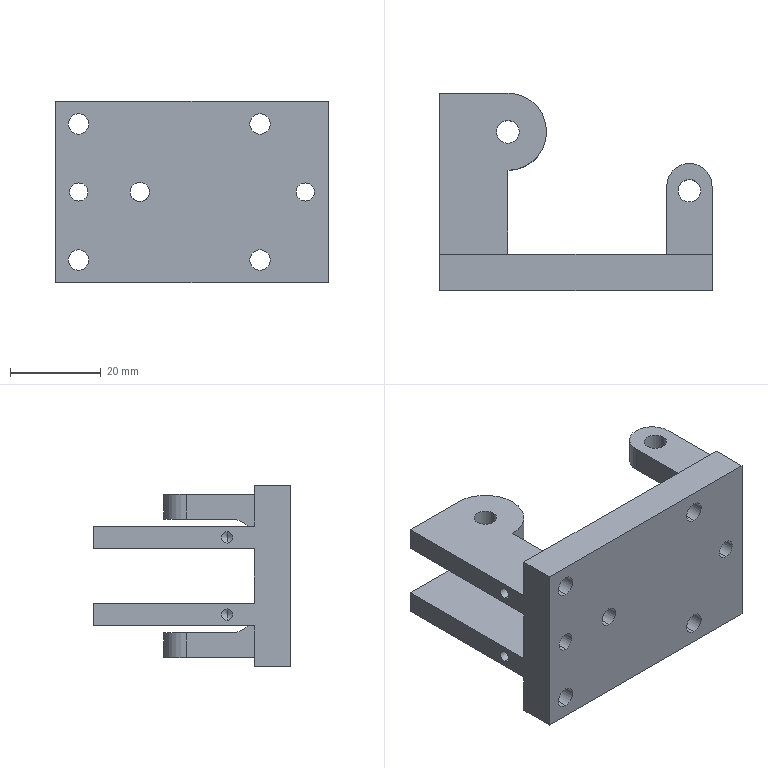Part | STEP file | X77b-01007 | 1 solid | 77 faces | box 60 x 43.5 x 40 mm | volume 25586 mm3 | cylinder 48 | plane 25 | cone 4 | commonest cylinder face diameters 4.5 x8 5 x8 8 x8 2.5 x6 10 x6 4 x4